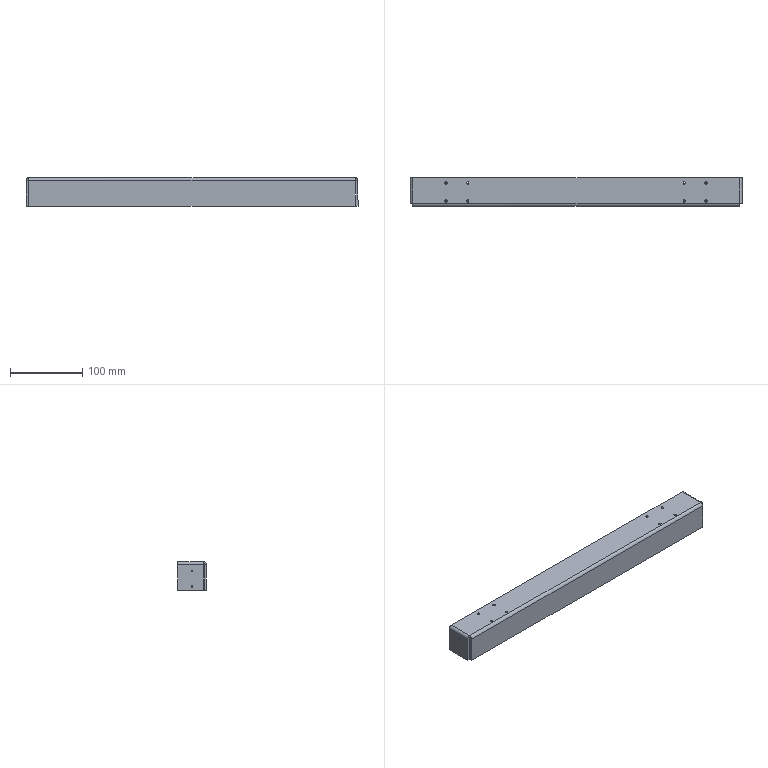Part | SolidWorks | features HoleWzd 2, EdgeFlange 1, FlatPattern 1, SMBaseFlange 1, SheetMetal 1 | 1 solid | 50 faces | box 460 x 40 x 40 mm | volume 111480 mm3 | cylinder 26 | plane 20 | spline 4 | commonest cylinder face diameters 3.3 x16 2.5 x4 2 x3 8 x3